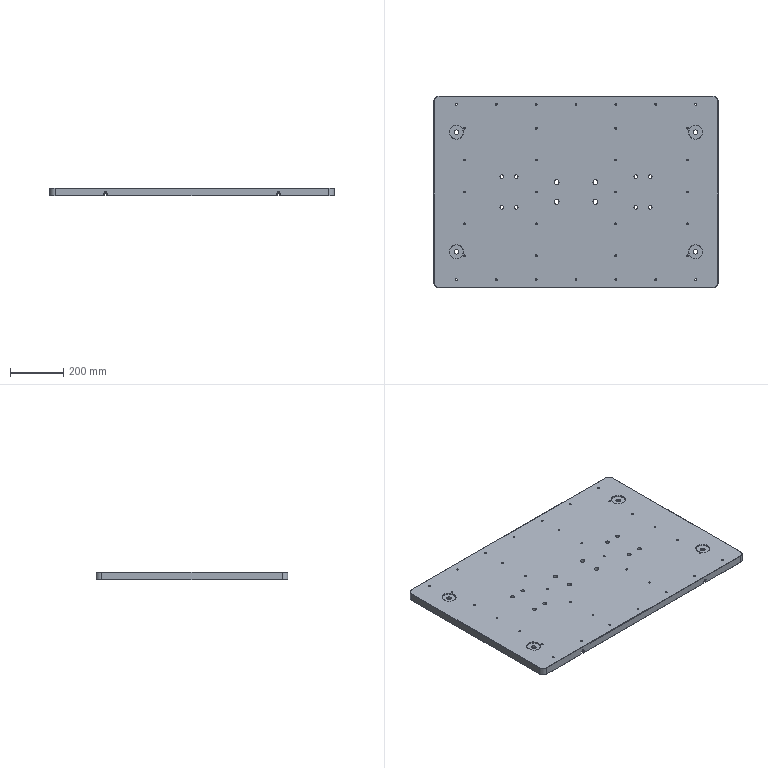Part | STEP file | TJ-DHQM-003-003 | 1 solid | 214 faces | box 1070 x 720 x 30 mm | volume 22699687 mm3 | cylinder 128 | plane 62 | cone 24 | commonest cylinder face diameters 6.8 x68 14 x16 17.5 x16 5 x8 26 x8 50 x8